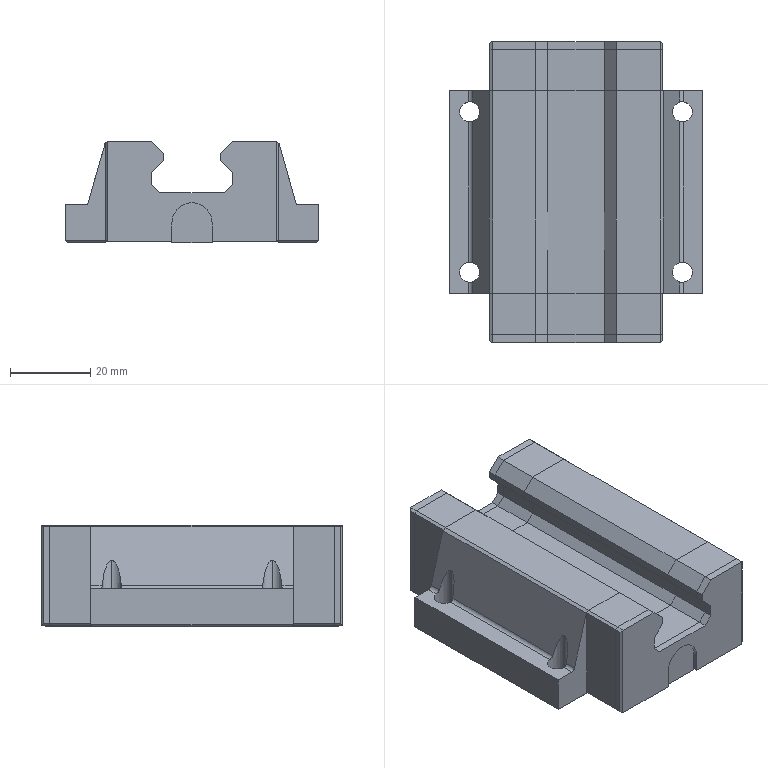Part | STEP file | HGW20CC | 3 solids | 167 faces | box 63 x 75 x 25.4 mm | volume 76452 mm3 | plane 150 | cylinder 17 | commonest cylinder face diameters 5 x8 2 x6 10 x3